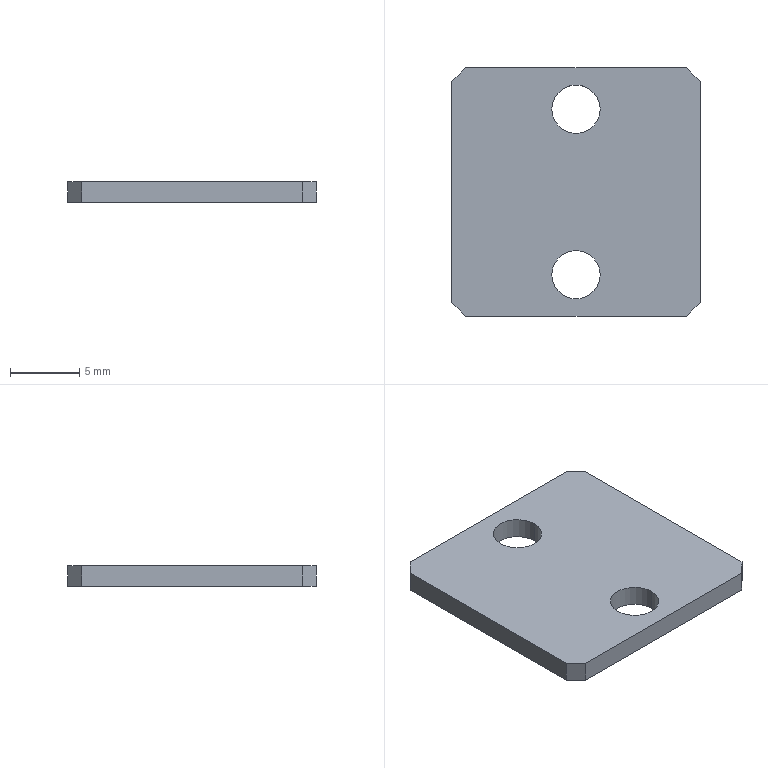Part | SolidWorks | features BaseBody 1 | 1 solid | 14 faces | box 18 x 18 x 1.5 mm | volume 454.137 mm3 | plane 10 | cylinder 4 | commonest cylinder face diameters 3.5 x4
STEP:
#1=CARTESIAN_POINT('',(7.25,3.,0.));
#2=VERTEX_POINT('',#1);
#3=CARTESIAN_POINT('',(10.75,3.,0.));
#4=VERTEX_POINT('',#3);
#5=CARTESIAN_POINT('',(9.,3.,0.));
#6=DIRECTION('',(0.,0.,1.));
#7=DIRECTION('',(1.,0.,0.));
#8=AXIS2_PLACEMENT_3D('',#5,#6,#7);
#9=CIRCLE('',#8,1.75);
#10=EDGE_CURVE('',#2,#4,#9,.T.);
#11=ORIENTED_EDGE('',*,*,#10,.F.);
#12=CARTESIAN_POINT('',(7.25,3.,1.5));
#13=VERTEX_POINT('',#12);
#14=CARTESIAN_POINT('',(7.25,3.,0.));
#15=DIRECTION('',(0.,0.,1.));
#16=VECTOR('',#15,1000.);
#17=LINE('',#14,#16);
#18=EDGE_CURVE('',#2,#13,#17,.T.);
#19=ORIENTED_EDGE('',*,*,#18,.T.);
#20=CARTESIAN_POINT('',(10.75,3.,1.5));
#21=VERTEX_POINT('',#20);
#22=CARTESIAN_POINT('',(9.,3.,1.5));
#23=DIRECTION('',(0.,0.,1.));
#24=DIRECTION('',(1.,0.,0.));
#25=AXIS2_PLACEMENT_3D('',#22,#23,#24);
#26=CIRCLE('',#25,1.75);
#27=EDGE_CURVE('',#13,#21,#26,.T.);
#28=ORIENTED_EDGE('',*,*,#27,.T.);
#29=CARTESIAN_POINT('',(10.75,3.,0.));
#30=DIRECTION('',(0.,0.,1.));
#31=VECTOR('',#30,1000.);
#32=LINE('',#29,#31);
#33=EDGE_CURVE('',#4,#21,#32,.T.);
#34=ORIENTED_EDGE('',*,*,#33,.F.);
#35=EDGE_LOOP('',(#11,#19,#28,#34));
#36=FACE_OUTER_BOUND('',#35,.T.);
#37=CARTESIAN_POINT('',(9.,3.,0.));
#38=DIRECTION('',(0.,0.,1.));
#39=DIRECTION('',(1.,0.,0.));
#40=AXIS2_PLACEMENT_3D('',#37,#38,#39);
#41=CYLINDRICAL_SURFACE('',#40,1.75);
#42=ADVANCED_FACE('',(#36),#41,.F.);
#43=CARTESIAN_POINT('',(7.25,15.,0.));
#44=VERTEX_POINT('',#43);
#45=CARTESIAN_POINT('',(10.75,15.,0.));
#46=VERTEX_POINT('',#45);
#47=CARTESIAN_POINT('',(9.,15.,0.));
#48=DIRECTION('',(0.,0.,1.));
#49=DIRECTION('',(1.,0.,0.));
#50=AXIS2_PLACEMENT_3D('',#47,#48,#49);
#51=CIRCLE('',#50,1.75);
#52=EDGE_CURVE('',#44,#46,#51,.T.);
#53=ORIENTED_EDGE('',*,*,#52,.F.);
#54=CARTESIAN_POINT('',(7.25,15.,1.5));
#55=VERTEX_POINT('',#54);
#56=CARTESIAN_POINT('',(7.25,15.,0.));
#57=DIRECTION('',(0.,0.,1.));
#58=VECTOR('',#57,1000.);
#59=LINE('',#56,#58);
#60=EDGE_CURVE('',#44,#55,#59,.T.);
#61=ORIENTED_EDGE('',*,*,#60,.T.);
#62=CARTESIAN_POINT('',(10.75,15.,1.5));
#63=VERTEX_POINT('',#62);
#64=CARTESIAN_POINT('',(9.,15.,1.5));
#65=DIRECTION('',(0.,0.,1.));
#66=DIRECTION('',(1.,0.,0.));
#67=AXIS2_PLACEMENT_3D('',#64,#65,#66);
#68=CIRCLE('',#67,1.75);
#69=EDGE_CURVE('',#55,#63,#68,.T.);
#70=ORIENTED_EDGE('',*,*,#69,.T.);
#71=CARTESIAN_POINT('',(10.75,15.,0.));
#72=DIRECTION('',(0.,0.,1.));
#73=VECTOR('',#72,1000.);
#74=LINE('',#71,#73);
#75=EDGE_CURVE('',#46,#63,#74,.T.);
#76=ORIENTED_EDGE('',*,*,#75,.F.);
#77=EDGE_LOOP('',(#53,#61,#70,#76));
#78=FACE_OUTER_BOUND('',#77,.T.);
#79=CARTESIAN_POINT('',(9.,15.,0.));
#80=DIRECTION('',(0.,0.,1.));
#81=DIRECTION('',(1.,0.,0.));
#82=AXIS2_PLACEMENT_3D('',#79,#80,#81);
#83=CYLINDRICAL_SURFACE('',#82,1.75);
#84=ADVANCED_FACE('',(#78),#83,.F.);
#85=CARTESIAN_POINT('',(17.,18.,1.5));
#86=VERTEX_POINT('',#85);
#87=CARTESIAN_POINT('',(18.,17.,1.5));
#88=VERTEX_POINT('',#87);
#89=CARTESIAN_POINT('',(17.,18.,1.5));
#90=DIRECTION('',(0.7071,-0.7071,0.));
#91=VECTOR('',#90,1000.);
#92=LINE('',#89,#91);
#93=EDGE_CURVE('',#86,#88,#92,.T.);
#94=ORIENTED_EDGE('',*,*,#93,.F.);
#95=CARTESIAN_POINT('',(1.,18.,1.5));
#96=VERTEX_POINT('',#95);
#97=CARTESIAN_POINT('',(0.,18.,1.5));
#98=DIRECTION('',(1.,0.,0.));
#99=VECTOR('',#98,1000.);
#100=LINE('',#97,#99);
#101=EDGE_CURVE('',#96,#86,#100,.T.);
#102=ORIENTED_EDGE('',*,*,#101,.F.);
#103=CARTESIAN_POINT('',(0.,17.,1.5));
#104=VERTEX_POINT('',#103);
#105=CARTESIAN_POINT('',(0.,17.,1.5));
#106=DIRECTION('',(0.7071,0.7071,0.));
#107=VECTOR('',#106,1000.);
#108=LINE('',#105,#107);
#109=EDGE_CURVE('',#104,#96,#108,.T.);
#110=ORIENTED_EDGE('',*,*,#109,.F.);
#111=CARTESIAN_POINT('',(0.,1.,1.5));
#112=VERTEX_POINT('',#111);
#113=CARTESIAN_POINT('',(0.,0.,1.5));
#114=DIRECTION('',(0.,1.,0.));
#115=VECTOR('',#114,1000.);
#116=LINE('',#113,#115);
#117=EDGE_CURVE('',#112,#104,#116,.T.);
#118=ORIENTED_EDGE('',*,*,#117,.F.);
#119=CARTESIAN_POINT('',(1.,0.,1.5));
#120=VERTEX_POINT('',#119);
#121=CARTESIAN_POINT('',(1.,0.,1.5));
#122=DIRECTION('',(-0.7071,0.7071,0.));
#123=VECTOR('',#122,1000.);
#124=LINE('',#121,#123);
#125=EDGE_CURVE('',#120,#112,#124,.T.);
#126=ORIENTED_EDGE('',*,*,#125,.F.);
#127=CARTESIAN_POINT('',(17.,0.,1.5));
#128=VERTEX_POINT('',#127);
#129=CARTESIAN_POINT('',(0.,0.,1.5));
#130=DIRECTION('',(-1.,0.,0.));
#131=VECTOR('',#130,1000.);
#132=LINE('',#129,#131);
#133=EDGE_CURVE('',#128,#120,#132,.T.);
#134=ORIENTED_EDGE('',*,*,#133,.F.);
#135=CARTESIAN_POINT('',(18.,1.,1.5));
#136=VERTEX_POINT('',#135);
#137=CARTESIAN_POINT('',(18.,1.,1.5));
#138=DIRECTION('',(-0.7071,-0.7071,0.));
#139=VECTOR('',#138,1000.);
#140=LINE('',#137,#139);
#141=EDGE_CURVE('',#136,#128,#140,.T.);
#142=ORIENTED_EDGE('',*,*,#141,.F.);
#143=CARTESIAN_POINT('',(18.,0.,1.5));
#144=DIRECTION('',(0.,-1.,0.));
#145=VECTOR('',#144,1000.);
#146=LINE('',#143,#145);
#147=EDGE_CURVE('',#88,#136,#146,.T.);
#148=ORIENTED_EDGE('',*,*,#147,.F.);
#149=EDGE_LOOP('',(#94,#102,#110,#118,#126,#134,#142,#148));
#150=FACE_OUTER_BOUND('',#149,.T.);
#151=CARTESIAN_POINT('',(9.,3.,1.5));
#152=DIRECTION('',(0.,0.,1.));
#153=DIRECTION('',(1.,0.,0.));
#154=AXIS2_PLACEMENT_3D('',#151,#152,#153);
#155=CIRCLE('',#154,1.75);
#156=EDGE_CURVE('',#21,#13,#155,.T.);
#157=ORIENTED_EDGE('',*,*,#156,.F.);
#158=ORIENTED_EDGE('',*,*,#27,.F.);
#159=EDGE_LOOP('',(#157,#158));
#160=FACE_BOUND('',#159,.T.);
#161=CARTESIAN_POINT('',(9.,15.,1.5));
#162=DIRECTION('',(0.,0.,1.));
#163=DIRECTION('',(1.,0.,0.));
#164=AXIS2_PLACEMENT_3D('',#161,#162,#163);
#165=CIRCLE('',#164,1.75);
#166=EDGE_CURVE('',#63,#55,#165,.T.);
#167=ORIENTED_EDGE('',*,*,#166,.F.);
#168=ORIENTED_EDGE('',*,*,#69,.F.);
#169=EDGE_LOOP('',(#167,#168));
#170=FACE_BOUND('',#169,.T.);
#171=CARTESIAN_POINT('',(0.,0.,1.5));
#172=DIRECTION('',(0.,0.,-1.));
#173=DIRECTION('',(-1.,0.,0.));
#174=AXIS2_PLACEMENT_3D('',#171,#172,#173);
#175=PLANE('',#174);
#176=ADVANCED_FACE('',(#150,#160,#170),#175,.F.);
#177=CARTESIAN_POINT('',(18.,17.,0.));
#178=VERTEX_POINT('',#177);
#179=CARTESIAN_POINT('',(18.,17.,1.5));
#180=DIRECTION('',(0.,0.,-1.));
#181=VECTOR('',#180,1000.);
#182=LINE('',#179,#181);
#183=EDGE_CURVE('',#88,#178,#182,.T.);
#184=ORIENTED_EDGE('',*,*,#183,.F.);
#185=ORIENTED_EDGE('',*,*,#147,.T.);
#186=CARTESIAN_POINT('',(18.,1.,0.));
#187=VERTEX_POINT('',#186);
#188=CARTESIAN_POINT('',(18.,1.,1.5));
#189=DIRECTION('',(0.,0.,1.));
#190=VECTOR('',#189,1000.);
#191=LINE('',#188,#190);
#192=EDGE_CURVE('',#187,#136,#191,.T.);
#193=ORIENTED_EDGE('',*,*,#192,.F.);
#194=CARTESIAN_POINT('',(18.,0.,0.));
#195=DIRECTION('',(0.,-1.,0.));
#196=VECTOR('',#195,1000.);
#197=LINE('',#194,#196);
#198=EDGE_CURVE('',#178,#187,#197,.T.);
#199=ORIENTED_EDGE('',*,*,#198,.F.);
#200=EDGE_LOOP('',(#184,#185,#193,#199));
#201=FACE_OUTER_BOUND('',#200,.T.);
#202=CARTESIAN_POINT('',(18.,0.,1.5));
#203=DIRECTION('',(-1.,0.,0.));
#204=DIRECTION('',(0.,0.,1.));
#205=AXIS2_PLACEMENT_3D('',#202,#203,#204);
#206=PLANE('',#205);
#207=ADVANCED_FACE('',(#201),#206,.F.);
#208=ORIENTED_EDGE('',*,*,#183,.T.);
#209=CARTESIAN_POINT('',(17.,18.,0.));
#210=VERTEX_POINT('',#209);
#211=CARTESIAN_POINT('',(17.,18.,0.));
#212=DIRECTION('',(0.7071,-0.7071,0.));
#213=VECTOR('',#212,1000.);
#214=LINE('',#211,#213);
#215=EDGE_CURVE('',#210,#178,#214,.T.);
#216=ORIENTED_EDGE('',*,*,#215,.F.);
#217=CARTESIAN_POINT('',(17.,18.,1.5));
#218=DIRECTION('',(0.,0.,-1.));
#219=VECTOR('',#218,1000.);
#220=LINE('',#217,#219);
#221=EDGE_CURVE('',#86,#210,#220,.T.);
#222=ORIENTED_EDGE('',*,*,#221,.F.);
#223=ORIENTED_EDGE('',*,*,#93,.T.);
#224=EDGE_LOOP('',(#208,#216,#222,#223));
#225=FACE_OUTER_BOUND('',#224,.T.);
#226=CARTESIAN_POINT('',(17.,18.,1.5));
#227=DIRECTION('',(-0.7071,-0.7071,0.));
#228=DIRECTION('',(0.7071,-0.7071,0.));
#229=AXIS2_PLACEMENT_3D('',#226,#227,#228);
#230=PLANE('',#229);
#231=ADVANCED_FACE('',(#225),#230,.F.);
#232=ORIENTED_EDGE('',*,*,#221,.T.);
#233=CARTESIAN_POINT('',(1.,18.,0.));
#234=VERTEX_POINT('',#233);
#235=CARTESIAN_POINT('',(0.,18.,0.));
#236=DIRECTION('',(1.,0.,0.));
#237=VECTOR('',#236,1000.);
#238=LINE('',#235,#237);
#239=EDGE_CURVE('',#234,#210,#238,.T.);
#240=ORIENTED_EDGE('',*,*,#239,.F.);
#241=CARTESIAN_POINT('',(1.,18.,1.5));
#242=DIRECTION('',(0.,0.,-1.));
#243=VECTOR('',#242,1000.);
#244=LINE('',#241,#243);
#245=EDGE_CURVE('',#96,#234,#244,.T.);
#246=ORIENTED_EDGE('',*,*,#245,.F.);
#247=ORIENTED_EDGE('',*,*,#101,.T.);
#248=EDGE_LOOP('',(#232,#240,#246,#247));
#249=FACE_OUTER_BOUND('',#248,.T.);
#250=CARTESIAN_POINT('',(0.,18.,1.5));
#251=DIRECTION('',(0.,-1.,0.));
#252=DIRECTION('',(0.,0.,-1.));
#253=AXIS2_PLACEMENT_3D('',#250,#251,#252);
#254=PLANE('',#253);
#255=ADVANCED_FACE('',(#249),#254,.F.);
#256=ORIENTED_EDGE('',*,*,#245,.T.);
#257=CARTESIAN_POINT('',(0.,17.,0.));
#258=VERTEX_POINT('',#257);
#259=CARTESIAN_POINT('',(0.,17.,0.));
#260=DIRECTION('',(0.7071,0.7071,0.));
#261=VECTOR('',#260,1000.);
#262=LINE('',#259,#261);
#263=EDGE_CURVE('',#258,#234,#262,.T.);
#264=ORIENTED_EDGE('',*,*,#263,.F.);
#265=CARTESIAN_POINT('',(0.,17.,1.5));
#266=DIRECTION('',(0.,0.,-1.));
#267=VECTOR('',#266,1000.);
#268=LINE('',#265,#267);
#269=EDGE_CURVE('',#104,#258,#268,.T.);
#270=ORIENTED_EDGE('',*,*,#269,.F.);
#271=ORIENTED_EDGE('',*,*,#109,.T.);
#272=EDGE_LOOP('',(#256,#264,#270,#271));
#273=FACE_OUTER_BOUND('',#272,.T.);
#274=CARTESIAN_POINT('',(0.,17.,1.5));
#275=DIRECTION('',(0.7071,-0.7071,0.));
#276=DIRECTION('',(0.7071,0.7071,0.));
#277=AXIS2_PLACEMENT_3D('',#274,#275,#276);
#278=PLANE('',#277);
#279=ADVANCED_FACE('',(#273),#278,.F.);
#280=ORIENTED_EDGE('',*,*,#269,.T.);
#281=CARTESIAN_POINT('',(0.,1.,0.));
#282=VERTEX_POINT('',#281);
#283=CARTESIAN_POINT('',(0.,0.,0.));
#284=DIRECTION('',(0.,1.,0.));
#285=VECTOR('',#284,1000.);
#286=LINE('',#283,#285);
#287=EDGE_CURVE('',#282,#258,#286,.T.);
#288=ORIENTED_EDGE('',*,*,#287,.F.);
#289=CARTESIAN_POINT('',(0.,1.,1.5));
#290=DIRECTION('',(0.,0.,-1.));
#291=VECTOR('',#290,1000.);
#292=LINE('',#289,#291);
#293=EDGE_CURVE('',#112,#282,#292,.T.);
#294=ORIENTED_EDGE('',*,*,#293,.F.);
#295=ORIENTED_EDGE('',*,*,#117,.T.);
#296=EDGE_LOOP('',(#280,#288,#294,#295));
#297=FACE_OUTER_BOUND('',#296,.T.);
#298=CARTESIAN_POINT('',(0.,0.,1.5));
#299=DIRECTION('',(1.,0.,0.));
#300=DIRECTION('',(0.,0.,-1.));
#301=AXIS2_PLACEMENT_3D('',#298,#299,#300);
#302=PLANE('',#301);
#303=ADVANCED_FACE('',(#297),#302,.F.);
#304=ORIENTED_EDGE('',*,*,#293,.T.);
#305=CARTESIAN_POINT('',(1.,0.,0.));
#306=VERTEX_POINT('',#305);
#307=CARTESIAN_POINT('',(1.,0.,0.));
#308=DIRECTION('',(-0.7071,0.7071,0.));
#309=VECTOR('',#308,1000.);
#310=LINE('',#307,#309);
#311=EDGE_CURVE('',#306,#282,#310,.T.);
#312=ORIENTED_EDGE('',*,*,#311,.F.);
#313=CARTESIAN_POINT('',(1.,0.,1.5));
#314=DIRECTION('',(0.,0.,-1.));
#315=VECTOR('',#314,1000.);
#316=LINE('',#313,#315);
#317=EDGE_CURVE('',#120,#306,#316,.T.);
#318=ORIENTED_EDGE('',*,*,#317,.F.);
#319=ORIENTED_EDGE('',*,*,#125,.T.);
#320=EDGE_LOOP('',(#304,#312,#318,#319));
#321=FACE_OUTER_BOUND('',#320,.T.);
#322=CARTESIAN_POINT('',(1.,0.,1.5));
#323=DIRECTION('',(0.7071,0.7071,0.));
#324=DIRECTION('',(-0.7071,0.7071,0.));
#325=AXIS2_PLACEMENT_3D('',#322,#323,#324);
#326=PLANE('',#325);
#327=ADVANCED_FACE('',(#321),#326,.F.);
#328=ORIENTED_EDGE('',*,*,#317,.T.);
#329=CARTESIAN_POINT('',(17.,0.,0.));
#330=VERTEX_POINT('',#329);
#331=CARTESIAN_POINT('',(0.,0.,0.));
#332=DIRECTION('',(-1.,0.,0.));
#333=VECTOR('',#332,1000.);
#334=LINE('',#331,#333);
#335=EDGE_CURVE('',#330,#306,#334,.T.);
#336=ORIENTED_EDGE('',*,*,#335,.F.);
#337=CARTESIAN_POINT('',(17.,0.,1.5));
#338=DIRECTION('',(0.,0.,-1.));
#339=VECTOR('',#338,1000.);
#340=LINE('',#337,#339);
#341=EDGE_CURVE('',#128,#330,#340,.T.);
#342=ORIENTED_EDGE('',*,*,#341,.F.);
#343=ORIENTED_EDGE('',*,*,#133,.T.);
#344=EDGE_LOOP('',(#328,#336,#342,#343));
#345=FACE_OUTER_BOUND('',#344,.T.);
#346=CARTESIAN_POINT('',(0.,0.,1.5));
#347=DIRECTION('',(0.,1.,0.));
#348=DIRECTION('',(0.,0.,1.));
#349=AXIS2_PLACEMENT_3D('',#346,#347,#348);
#350=PLANE('',#349);
#351=ADVANCED_FACE('',(#345),#350,.F.);
#352=ORIENTED_EDGE('',*,*,#341,.T.);
#353=CARTESIAN_POINT('',(18.,1.,0.));
#354=DIRECTION('',(-0.7071,-0.7071,0.));
#355=VECTOR('',#354,1000.);
#356=LINE('',#353,#355);
#357=EDGE_CURVE('',#187,#330,#356,.T.);
#358=ORIENTED_EDGE('',*,*,#357,.F.);
#359=ORIENTED_EDGE('',*,*,#192,.T.);
#360=ORIENTED_EDGE('',*,*,#141,.T.);
#361=EDGE_LOOP('',(#352,#358,#359,#360));
#362=FACE_OUTER_BOUND('',#361,.T.);
#363=CARTESIAN_POINT('',(18.,1.,1.5));
#364=DIRECTION('',(-0.7071,0.7071,0.));
#365=DIRECTION('',(-0.7071,-0.7071,0.));
#366=AXIS2_PLACEMENT_3D('',#363,#364,#365);
#367=PLANE('',#366);
#368=ADVANCED_FACE('',(#362),#367,.F.);
#369=ORIENTED_EDGE('',*,*,#18,.F.);
#370=CARTESIAN_POINT('',(9.,3.,0.));
#371=DIRECTION('',(0.,0.,1.));
#372=DIRECTION('',(1.,0.,0.));
#373=AXIS2_PLACEMENT_3D('',#370,#371,#372);
#374=CIRCLE('',#373,1.75);
#375=EDGE_CURVE('',#4,#2,#374,.T.);
#376=ORIENTED_EDGE('',*,*,#375,.F.);
#377=ORIENTED_EDGE('',*,*,#33,.T.);
#378=ORIENTED_EDGE('',*,*,#156,.T.);
#379=EDGE_LOOP('',(#369,#376,#377,#378));
#380=FACE_OUTER_BOUND('',#379,.T.);
#381=CARTESIAN_POINT('',(9.,3.,0.));
#382=DIRECTION('',(0.,0.,1.));
#383=DIRECTION('',(1.,0.,0.));
#384=AXIS2_PLACEMENT_3D('',#381,#382,#383);
#385=CYLINDRICAL_SURFACE('',#384,1.75);
#386=ADVANCED_FACE('',(#380),#385,.F.);
#387=ORIENTED_EDGE('',*,*,#60,.F.);
#388=CARTESIAN_POINT('',(9.,15.,0.));
#389=DIRECTION('',(0.,0.,1.));
#390=DIRECTION('',(1.,0.,0.));
#391=AXIS2_PLACEMENT_3D('',#388,#389,#390);
#392=CIRCLE('',#391,1.75);
#393=EDGE_CURVE('',#46,#44,#392,.T.);
#394=ORIENTED_EDGE('',*,*,#393,.F.);
#395=ORIENTED_EDGE('',*,*,#75,.T.);
#396=ORIENTED_EDGE('',*,*,#166,.T.);
#397=EDGE_LOOP('',(#387,#394,#395,#396));
#398=FACE_OUTER_BOUND('',#397,.T.);
#399=CARTESIAN_POINT('',(9.,15.,0.));
#400=DIRECTION('',(0.,0.,1.));
#401=DIRECTION('',(1.,0.,0.));
#402=AXIS2_PLACEMENT_3D('',#399,#400,#401);
#403=CYLINDRICAL_SURFACE('',#402,1.75);
#404=ADVANCED_FACE('',(#398),#403,.F.);
#405=ORIENTED_EDGE('',*,*,#287,.T.);
#406=ORIENTED_EDGE('',*,*,#263,.T.);
#407=ORIENTED_EDGE('',*,*,#239,.T.);
#408=ORIENTED_EDGE('',*,*,#215,.T.);
#409=ORIENTED_EDGE('',*,*,#198,.T.);
#410=ORIENTED_EDGE('',*,*,#357,.T.);
#411=ORIENTED_EDGE('',*,*,#335,.T.);
#412=ORIENTED_EDGE('',*,*,#311,.T.);
#413=EDGE_LOOP('',(#405,#406,#407,#408,#409,#410,#411,#412));
#414=FACE_OUTER_BOUND('',#413,.T.);
#415=ORIENTED_EDGE('',*,*,#375,.T.);
#416=ORIENTED_EDGE('',*,*,#10,.T.);
#417=EDGE_LOOP('',(#415,#416));
#418=FACE_BOUND('',#417,.T.);
#419=ORIENTED_EDGE('',*,*,#393,.T.);
#420=ORIENTED_EDGE('',*,*,#52,.T.);
#421=EDGE_LOOP('',(#419,#420));
#422=FACE_BOUND('',#421,.T.);
#423=CARTESIAN_POINT('',(0.,0.,0.));
#424=DIRECTION('',(0.,0.,-1.));
#425=DIRECTION('',(-1.,0.,0.));
#426=AXIS2_PLACEMENT_3D('',#423,#424,#425);
#427=PLANE('',#426);
#428=ADVANCED_FACE('',(#414,#418,#422),#427,.T.);
#429=CLOSED_SHELL('',(#42,#84,#176,#207,#231,#255,#279,#303,#327,#351,#368,#386,#404,#428));
#430=MANIFOLD_SOLID_BREP('',#429);
#431=CARTESIAN_POINT('',(0.,0.,0.));
#432=DIRECTION('',(0.,0.,1.));
#433=DIRECTION('',(1.,0.,0.));
#434=AXIS2_PLACEMENT_3D('',#431,#432,#433);
#435=(LENGTH_UNIT()NAMED_UNIT(*)SI_UNIT(.MILLI.,.METRE.));
#436=UNCERTAINTY_MEASURE_WITH_UNIT(LENGTH_MEASURE(0.00001),#435,'','');
#437=(NAMED_UNIT(*)PLANE_ANGLE_UNIT()SI_UNIT($,.RADIAN.));
#438=(NAMED_UNIT(*)SI_UNIT($,.STERADIAN.)SOLID_ANGLE_UNIT());
#439=(GEOMETRIC_REPRESENTATION_CONTEXT(3)GLOBAL_UNCERTAINTY_ASSIGNED_CONTEXT((#436))GLOBAL_UNIT_ASSIGNED_CONTEXT((#435,#437,#438))REPRESENTATION_CONTEXT('',''));
#440=ADVANCED_BREP_SHAPE_REPRESENTATION('',(#430,#434),#439);